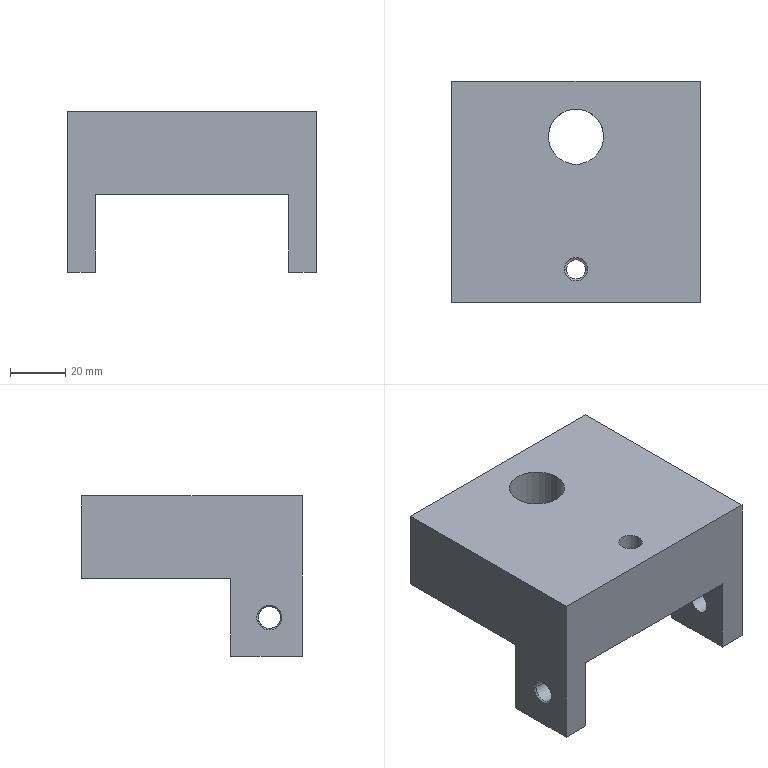Part | STEP file | BCC3 H14_1B | 1 solid | 26 faces | box 90 x 80 x 58 mm | volume 218426 mm3 | plane 12 | cylinder 8 | cone 6 | commonest cylinder face diameters 8 x4 8.5 x2 20 x2